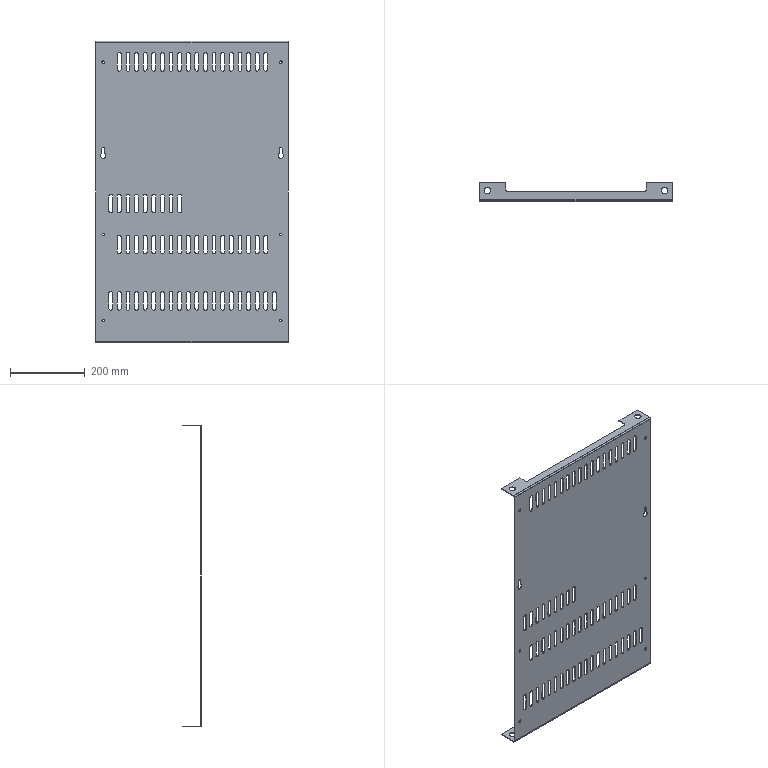Part | STEP file | 68352118 | 1 solid | 322 faces | box 514 x 50 x 805 mm | volume 820655 mm3 | cylinder 162 | plane 160 | commonest cylinder face diameters 10 x130 7 x14 17 x8 8 x6 4 x2 14 x2